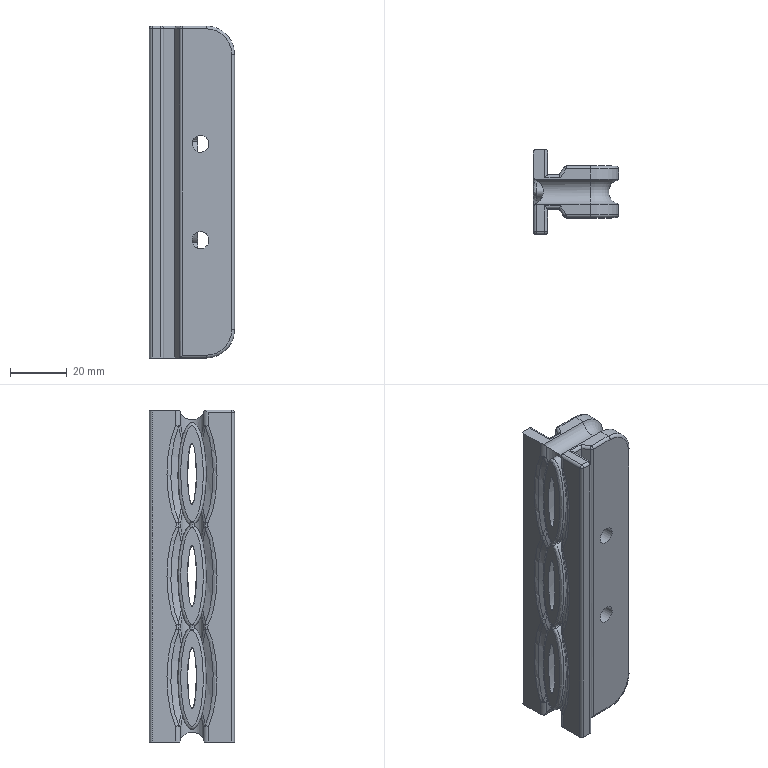Part | STEP file | jianzhendian | 1 solid | 143 faces | box 30 x 30 x 117 mm | volume 56101 mm3 | spline 51 | cylinder 50 | plane 23 | torus 10 | sphere 9 | commonest cylinder face diameters 2 x23 9 x9 0.919 x8 4 x4 20 x4 6 x2